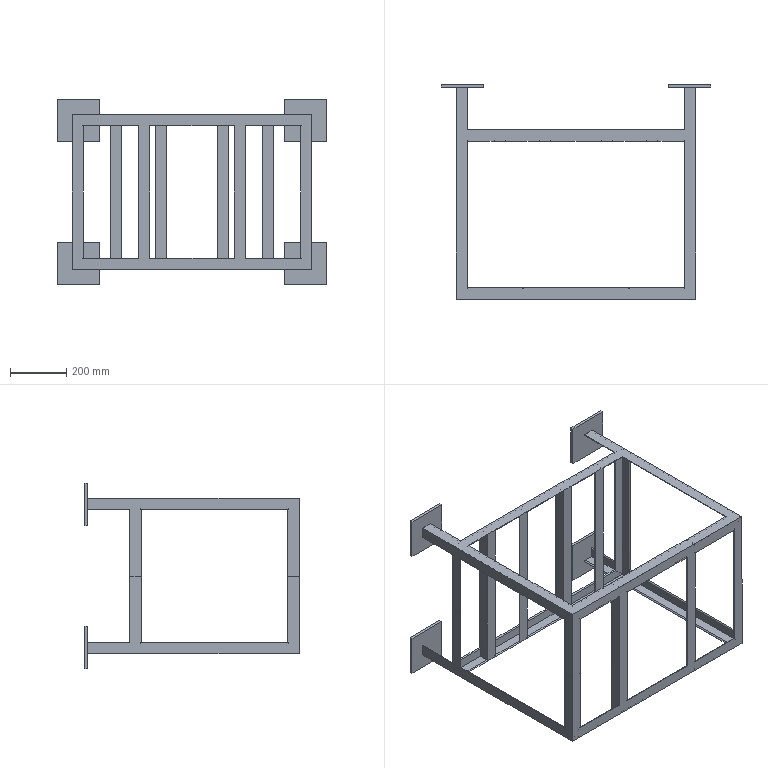Part | SolidWorks | features ICE 4, MirrorSolid 1, Sweep 1 | 1 solid | 171 faces | box 956 x 760 x 656 mm | volume 4250564 mm3 | plane 99 | cylinder 72 | commonest cylinder face diameters 8 x72